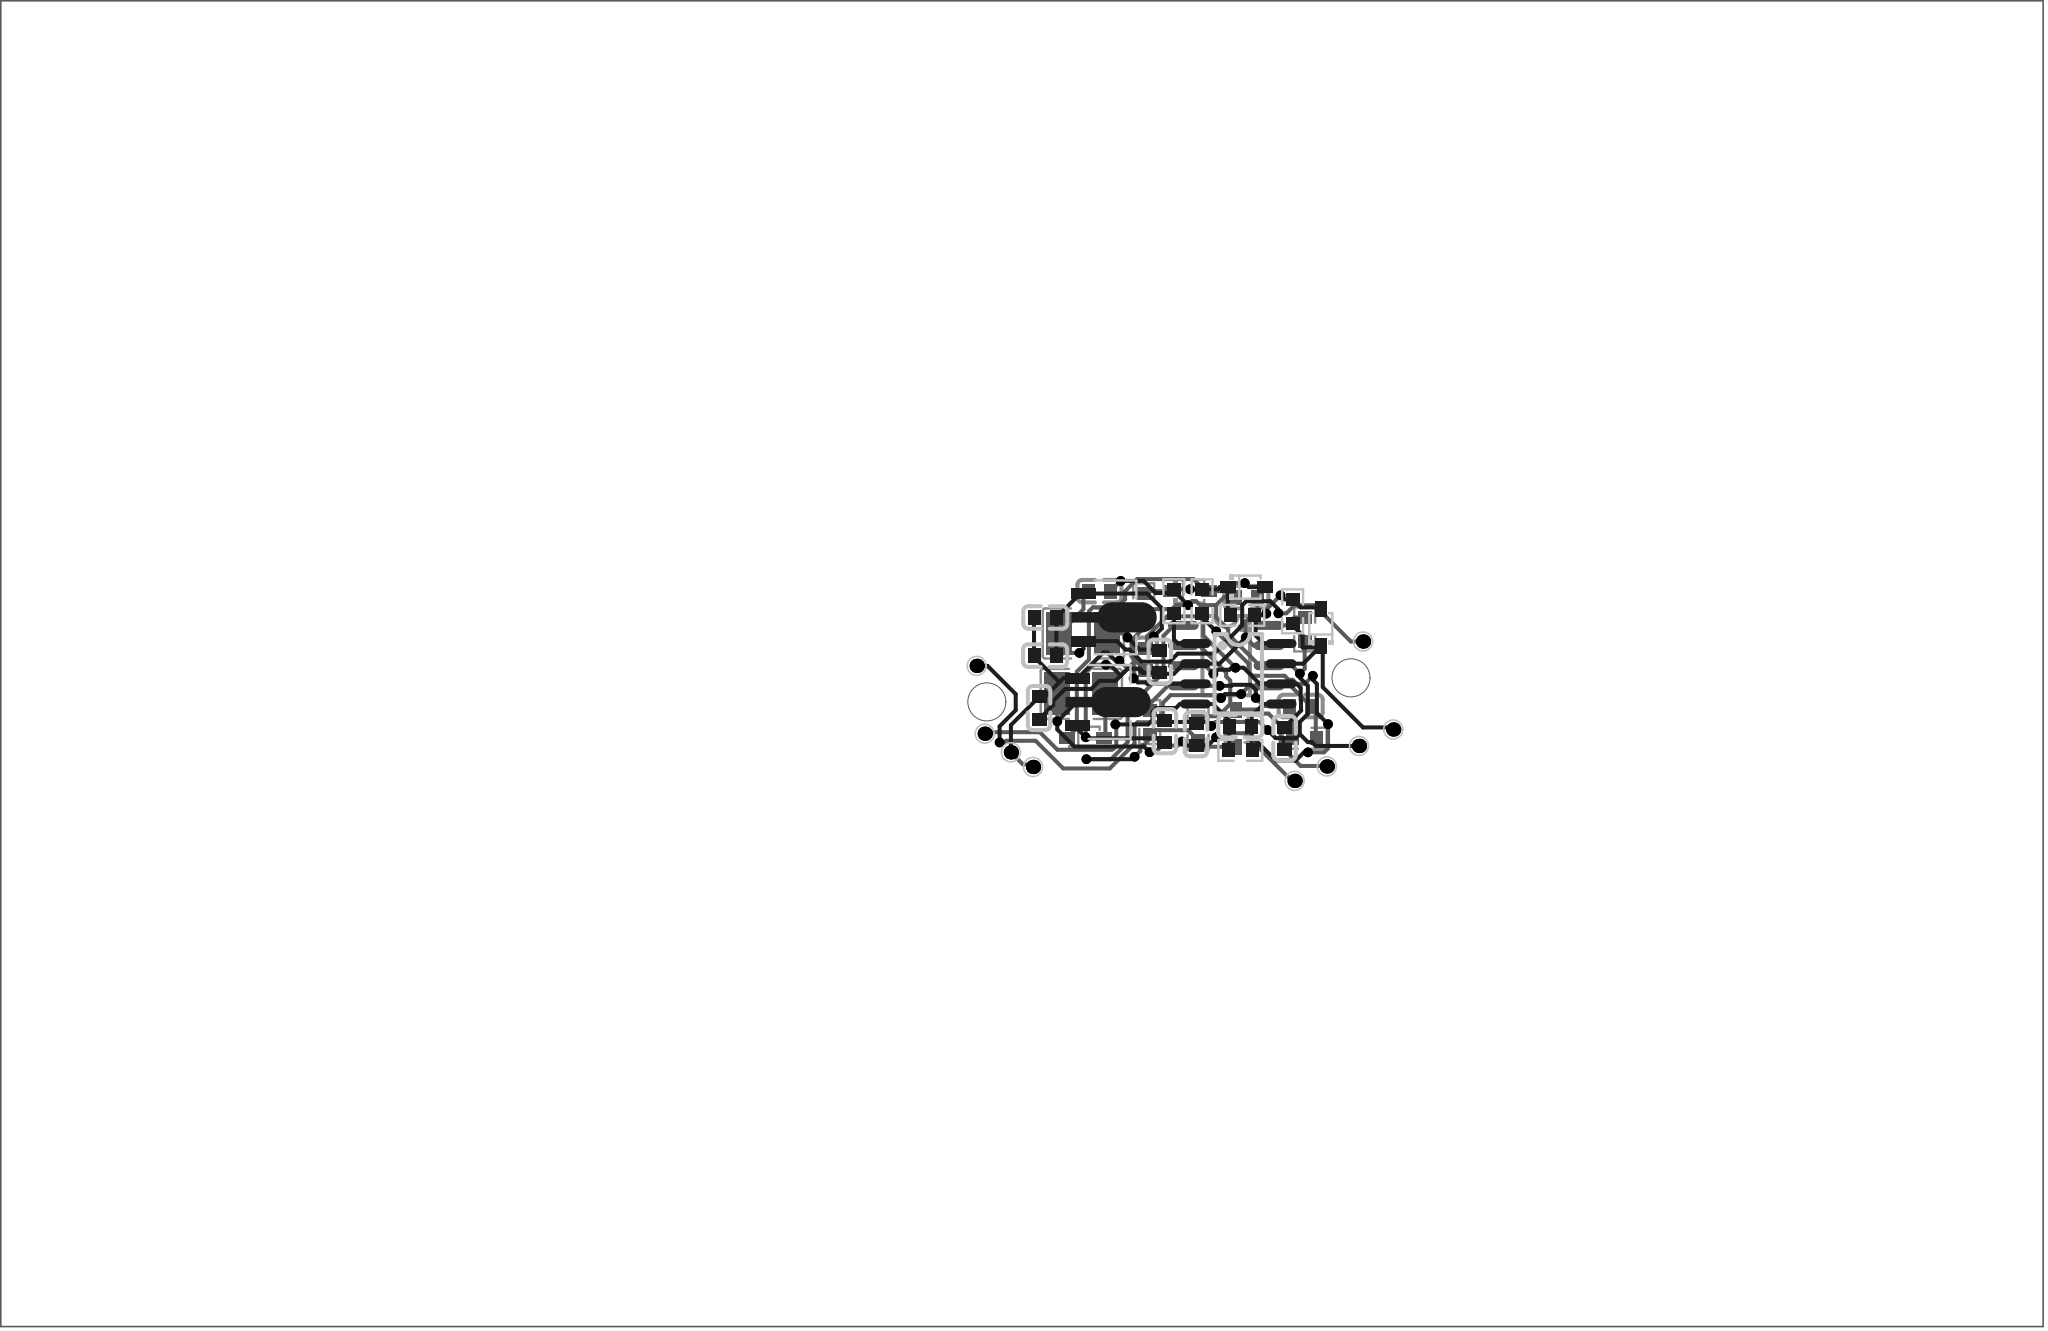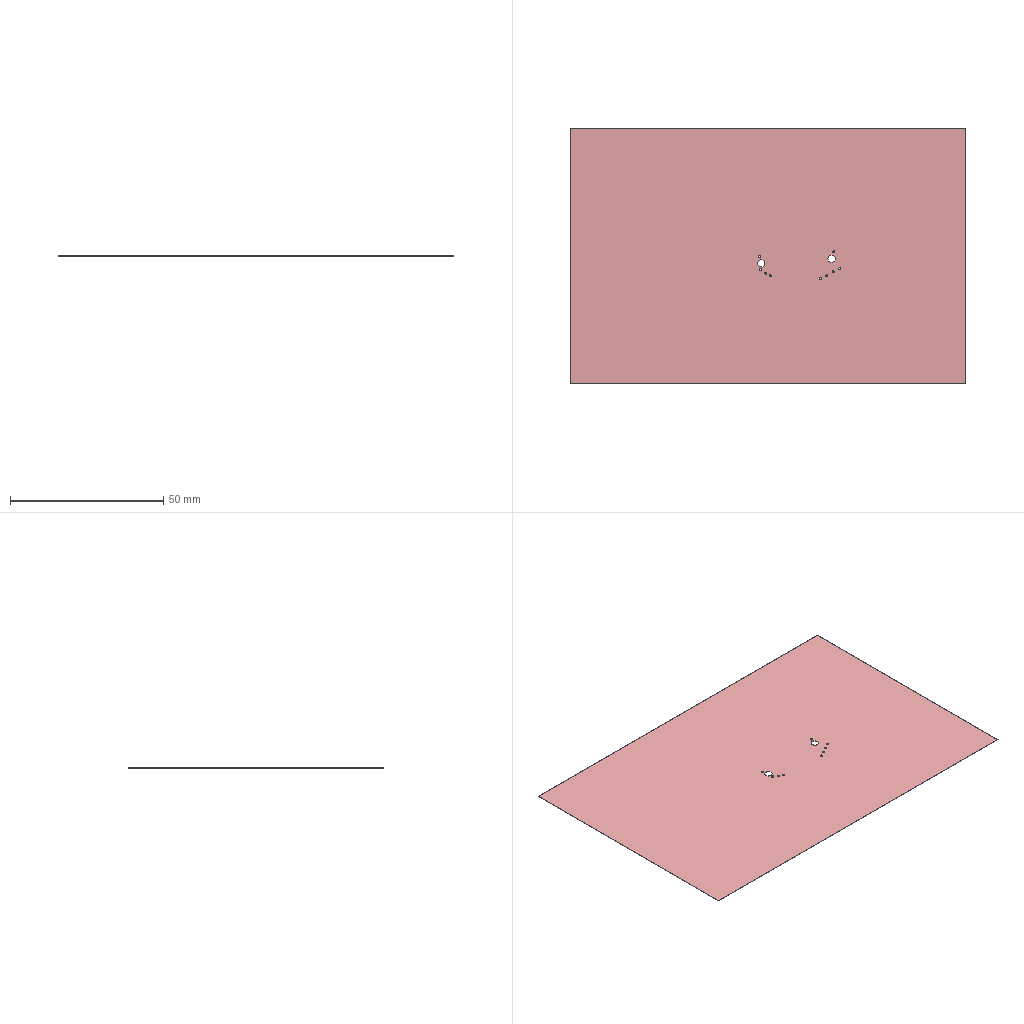Circuit board layout | Altium Designer | box 128.9 x 83.6 x 0.1 mm
Layer stack:
# Altium Designer layer stack of  (unit mm; dielectric type: 0 none, 1 core, 2 prepreg, 3 surface material)
index,name,kind,layer,copper_thickness_mm,dielectric_type,dielectric_thickness_mm,dielectric_material,dielectric_constant
0,Top Paste Mask Layer,other,,,,,,
1,Top Silkscreen Layer,other,,,,,,
2,Top Solder Mask Layer,dielectric,,,3,0.01,,3.3
3,Top Layer,copper,Top Layer,0.035,,,,
4,Bottom Layer,copper,Bottom Layer,0.035,,,,
5,Bottom Solder Mask Layer,dielectric,,,3,0.01,,3.3
6,Bottom Silkscreen Layer,other,,,,,,
7,Bottom Paste Mask Layer,other,,,,,,
# drill layer pairs: low layer,high layer
drill_pair,Top Layer,Bottom Layer
Part placement:
Designator,Comment,Layer,Footprint,Center-X(mm),Center-Y(mm),Rotation
C1,47nF,TopLayer,C0603,150.876,106.934,90
C2,47nF,TopLayer,C0603,143.002,111.76,270
C3,47nF,BottomLayer,C0603,142.113,111.887,90
C4,47nF,BottomLayer,C0603,148.463,115.824,0
C5,33pF,TopLayer,C0603,148.082,107.696,0
C6,33pF,BottomLayer,C0603,151.892,108.966,180
C7,100nF,BottomLayer,C0603,139.192,116.205,180
C8,100nF,TopLayer,C0603,145.288,107.188,270
C9,330nF,TopLayer,C0603,135.774,114.546,0
C10,330nF,TopLayer,C0603,143.321,107.377,270
C11,1uF,TopLayer,C0603,135.763,112.141,0
C12,1uF,TopLayer,C0603,135.382,108.839,270
C13,22uF,BottomLayer,C1210,138.176,113.538,0
C14,22uF,BottomLayer,C1210,138.049,109.728,0
D1,1N4148WS-7-F,TopLayer,SOD-323_L1.8-W1.3-LS2.5-RD,148.463,116.459,0
D2,1N4148WS-7-F,BottomLayer,SOD-323_L1.8-W1.3-LS2.5-RD,144.907,116.205,0
D3,1N4148WS-7-F,BottomLayer,SOD-323_L1.8-W1.3-LS2.5-RD,138.303,106.934,0
D4,1N4148WS-7-F,TopLayer,SOD-323_L1.8-W1.3-LS2.5-RD,153.162,113.919,90
D5,1N4148WS-7-F,BottomLayer,SOD-323_L1.8-W1.3-LS2.5-RD,147.828,107.569,270
R1,1.5M,TopLayer,R0603,148.082,106.172,0
R2,1.5M,BottomLayer,R0603,152.146,106.934,180
R3,205K,TopLayer,R0603,151.384,114.935,270
R4,4.7K,TopLayer,R0603,145.669,115.57,90
R5,200K,BottomLayer,R0603,145.415,107.569,90
R6,20K,BottomLayer,R0603,141.986,115.316,90
R7,33K,TopLayer,R0603,148.209,114.681,0
R8,33R,TopLayer,R0603,143.891,115.57,90
R9,33R,BottomLayer,R0603,152.146,113.792,270
R10,11K,BottomLayer,R0603,142.367,107.95,270
U1,LT1057IS8#PBF,TopLayer,SOIC-8_L5.0-W4.0-P1.27-LS6.0-BL,147.955,110.998,270
U2,LT1057IS8#PBF,BottomLayer,SOIC-8_L5.0-W4.0-P1.27-LS6.0-BL,147.193,112.141,270
U3,L78L12ABUTR,TopLayer,SOT-89-3_L4.5-W2.5-P1.50-LS4.2-BR,139.378,114.554,180
U4,L79L12ACUTR,TopLayer,SOT-89-3_L4.5-W2.5-P1.50-LS4.2-TL,138.997,109.22,0
U5,MTBD1-D011000,TopLayer,CR100,131.953,107.221,0
U6,MTBD1-D011000,TopLayer,CR100,133.604,106.045,0
U7,MTBD1-D011000,TopLayer,CR100,131.445,111.495,0
U8,MTBD1-D011000,TopLayer,CR100,135.001,105.123,0
U9,MTBD1-D011000,TopLayer,CR100,157.734,107.486,0
U10,MTBD1-D011000,TopLayer,CR100,155.575,106.448,0
U11,MTBD1-D011000,TopLayer,CR100,153.543,105.156,0
U12,MTBD1-D011000,TopLayer,CR100,151.511,104.245,0
U13,MTBD1-D011000,TopLayer,CR100,155.829,113.03,0
Pad and via stacks:
# Altium Designer via and pad stacks of  (unit mm). Each distinct definition once, with the count of objects using it.
# via: kind,start_layer,end_layer,hole_mm,diameter_mm,mode(0 simple;1 top-mid-bottom;2 full stack),diameter_per_layer,count,example_net
# pad: kind,layer,hole_mm,hole_type(0 round;1 square;2 slot),plating,top_size,top_shape(1 round;2 rect;3 octagon;9 rounded rect),mid_size,bottom_size,mode,footprint,size_per_layer,count,example
pad,Top Layer,0,0,plated,0.8x0.9,2,0.8x0.9,0.8x0.9,0,C0603,,16,C1.2
pad,Top Layer,0,0,plated,1x0.75,2,1x0.75,1x0.75,0,SOD-323_L1.8-W1.3-LS2.5-RD,,4,D1.2
pad,Top Layer,0,0,plated,0.8065x0.864,2,0.8065x0.864,0.8065x0.864,0,R0603,,10,R1.2
pad,Top Layer,0,0,plated,0.5684x1.95,1,0.5684x1.95,0.5684x1.95,0,SOIC-8_L5.0-W4.0-P1.27-LS6.0-BL,,8,U1.1
pad,Top Layer,0,0,plated,1.575x0.672,2,1.575x0.672,1.575x0.672,0,SOT-89-3_L4.5-W2.5-P1.50-LS4.2-BR,,2,U3.1
pad,Top Layer,0,0,plated,0.95x0.95,1,0.95x0.95,0.95x0.95,0,SOT-89-3_L4.5-W2.5-P1.50-LS4.2-BR,,1,U3.2
pad,Top Layer,0,0,plated,0.95x0.95,1,0.95x0.95,0.95x0.95,0,SOT-89-3_L4.5-W2.5-P1.50-LS4.2-TL,,1,U4.2
pad,Top Layer,0,0,plated,1.575x0.672,2,1.575x0.672,1.575x0.672,0,SOT-89-3_L4.5-W2.5-P1.50-LS4.2-TL,,2,U4.3
pad,Bottom Layer,0,0,plated,0.8x0.9,2,0.8x0.9,0.8x0.9,0,C0603,,8,C3.2
pad,Bottom Layer,0,0,plated,1.635x2.7,2,1.635x2.7,1.635x2.7,0,C1210,,4,C13.2
pad,Bottom Layer,0,0,plated,1x0.75,2,1x0.75,1x0.75,0,SOD-323_L1.8-W1.3-LS2.5-RD,,6,D2.2
pad,Bottom Layer,0,0,plated,0.8065x0.864,2,0.8065x0.864,0.8065x0.864,0,R0603,,10,R2.2
pad,Bottom Layer,0,0,plated,0.5684x1.95,1,0.5684x1.95,0.5684x1.95,0,SOIC-8_L5.0-W4.0-P1.27-LS6.0-BL,,8,U2.1
pad,Multi-Layer,0.7,0,plated,0.9x0.9,1,0.9x0.9,0.9x0.9,0,CR100,,9,U5.1
via,Top Layer,Bottom Layer,0.3048,0.61,0,,36,D1_1
Design rules, without the lines most boards share:
# Altium Designer design rules of  (exported by Altium Designer, unit mm)
# columns: name | kind | enabled | priority | scope1 | scope2 | descriptor | typed fields (field=value)
Default | 0 | enabled | 1 | All | All | Clearance Constraint (Gap=6mil) (All),(All) | gap=0.1524
Default_1 | 63 | enabled | 1 | All | All | Board Clearance Constraint (Gap=0mil) (All) |
otherClearance | 52 | enabled | 1 | All | All | Hole To Hole Clearance (Gap=11.8mil) (All),(All) | gap=0.2997
Default_2 | 2 | enabled | 1 | All | All | Width Constraint (Min=10mil) (Max=1000mil) (Preferred=10mil) (All) |
differentialPair | 51 | enabled | 1 | All | All | Differential Pairs Uncoupled Length using the Gap Constraints (Min=5mil) (Max=6mil) (Prefered=6mil)  and Width Constraints (Min=5mil) (Max=100mil) (Prefered=100mil) (All) |
Default_3 | 11 | enabled | 1 | All | All | Routing Via (MinHoleWidth=12mil) (MaxHoleWidth=1181mil) (PreferredHoleWidth=12mil) (MinWidth=24mil) (MaxWidth=1969mil) (PreferedWidth=24mil) (All) | via_min_hole=0.3048 via_max_hole=29.997 via_preferred_diameter=0.6096 via_preferred_hole=0.3048
Common | 13 | enabled | 2 | All | All | Solder Mask Expansion (Expansion =2mil) (All) | expansion=0.0508
Common_1 | 13 | enabled | 1 | IsVia | All | Solder Mask Expansion (Expansion =-1000mil) (IsVia) | expansion=-25.4